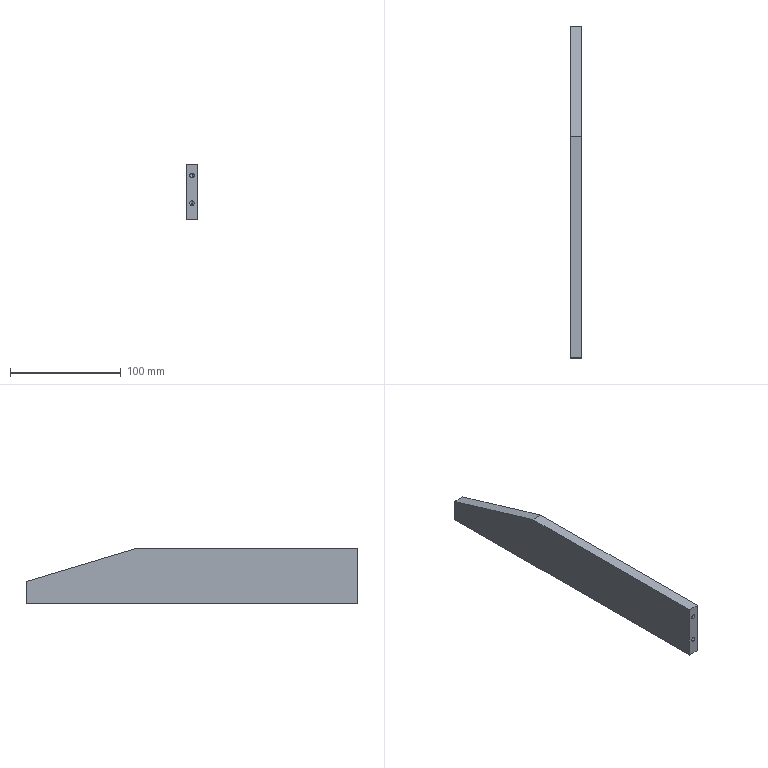Part | STEP file | 09-36 Support plate reinforcement plate | 1 solid | 31 faces | box 10 x 300 x 50 mm | volume 133768 mm3 | cylinder 12 | cone 12 | plane 7 | commonest cylinder face diameters 4.2 x12